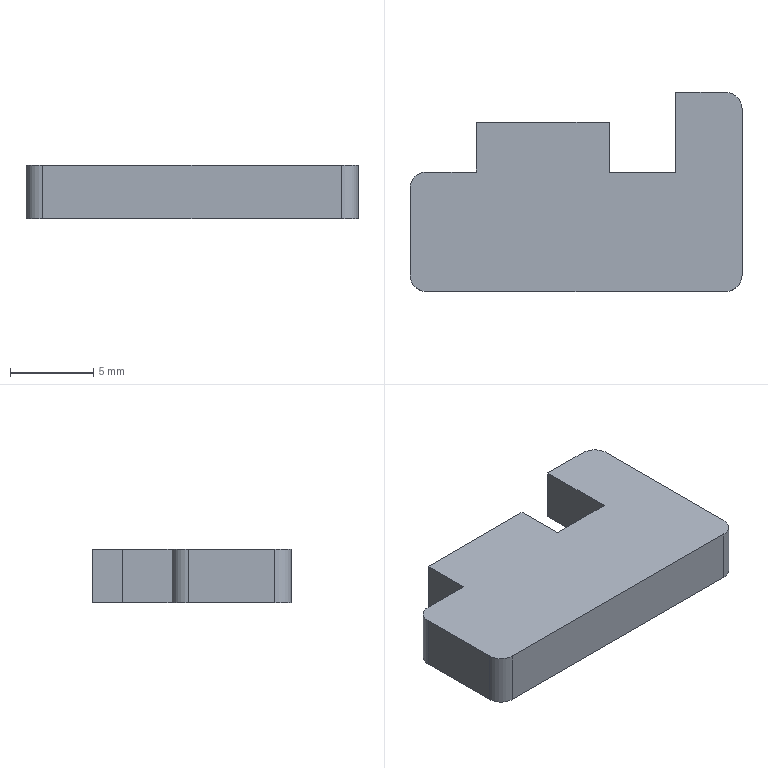Part | SolidWorks | features FlatPattern 1, SMBaseFlange 1, SheetMetal 1 | 1 solid | 16 faces | box 20 x 12 x 3.2 mm | volume 596.293 mm3 | plane 12 | cylinder 4 | commonest cylinder face diameters 2 x4
STEP:
#1=CARTESIAN_POINT('',(7.294,-19.84,0.));
#2=VERTEX_POINT('',#1);
#3=CARTESIAN_POINT('',(4.294,-19.84,0.));
#4=VERTEX_POINT('',#3);
#5=CARTESIAN_POINT('',(7.294,-19.84,0.));
#6=DIRECTION('',(-1.,0.,0.));
#7=VECTOR('',#6,1000.);
#8=LINE('',#5,#7);
#9=EDGE_CURVE('',#2,#4,#8,.T.);
#10=ORIENTED_EDGE('',*,*,#9,.F.);
#11=CARTESIAN_POINT('',(7.294,-19.84,-3.2));
#12=VERTEX_POINT('',#11);
#13=CARTESIAN_POINT('',(7.294,-19.84,-3.2));
#14=DIRECTION('',(0.,0.,1.));
#15=VECTOR('',#14,1000.);
#16=LINE('',#13,#15);
#17=EDGE_CURVE('',#12,#2,#16,.T.);
#18=ORIENTED_EDGE('',*,*,#17,.F.);
#19=CARTESIAN_POINT('',(4.294,-19.84,-3.2));
#20=VERTEX_POINT('',#19);
#21=CARTESIAN_POINT('',(7.294,-19.84,-3.2));
#22=DIRECTION('',(-1.,0.,0.));
#23=VECTOR('',#22,1000.);
#24=LINE('',#21,#23);
#25=EDGE_CURVE('',#12,#20,#24,.T.);
#26=ORIENTED_EDGE('',*,*,#25,.T.);
#27=CARTESIAN_POINT('',(4.294,-19.84,-3.2));
#28=DIRECTION('',(0.,0.,1.));
#29=VECTOR('',#28,1000.);
#30=LINE('',#27,#29);
#31=EDGE_CURVE('',#20,#4,#30,.T.);
#32=ORIENTED_EDGE('',*,*,#31,.T.);
#33=EDGE_LOOP('',(#10,#18,#26,#32));
#34=FACE_OUTER_BOUND('',#33,.T.);
#35=CARTESIAN_POINT('',(7.294,-19.84,-3.2));
#36=DIRECTION('',(0.,1.,0.));
#37=DIRECTION('',(-1.,0.,0.));
#38=AXIS2_PLACEMENT_3D('',#35,#36,#37);
#39=PLANE('',#38);
#40=ADVANCED_FACE('',(#34),#39,.T.);
#41=CARTESIAN_POINT('',(7.294,-16.84,0.));
#42=VERTEX_POINT('',#41);
#43=CARTESIAN_POINT('',(7.294,-19.84,0.));
#44=DIRECTION('',(0.,-1.,0.));
#45=VECTOR('',#44,1000.);
#46=LINE('',#43,#45);
#47=EDGE_CURVE('',#42,#2,#46,.T.);
#48=ORIENTED_EDGE('',*,*,#47,.F.);
#49=CARTESIAN_POINT('',(7.294,-16.84,-3.2));
#50=VERTEX_POINT('',#49);
#51=CARTESIAN_POINT('',(7.294,-16.84,-3.2));
#52=DIRECTION('',(0.,0.,1.));
#53=VECTOR('',#52,1000.);
#54=LINE('',#51,#53);
#55=EDGE_CURVE('',#50,#42,#54,.T.);
#56=ORIENTED_EDGE('',*,*,#55,.F.);
#57=CARTESIAN_POINT('',(7.294,-19.84,-3.2));
#58=DIRECTION('',(0.,-1.,0.));
#59=VECTOR('',#58,1000.);
#60=LINE('',#57,#59);
#61=EDGE_CURVE('',#50,#12,#60,.T.);
#62=ORIENTED_EDGE('',*,*,#61,.T.);
#63=ORIENTED_EDGE('',*,*,#17,.T.);
#64=EDGE_LOOP('',(#48,#56,#62,#63));
#65=FACE_OUTER_BOUND('',#64,.T.);
#66=CARTESIAN_POINT('',(7.294,-19.84,-3.2));
#67=DIRECTION('',(-1.,0.,0.));
#68=DIRECTION('',(0.,-1.,0.));
#69=AXIS2_PLACEMENT_3D('',#66,#67,#68);
#70=PLANE('',#69);
#71=ADVANCED_FACE('',(#65),#70,.T.);
#72=CARTESIAN_POINT('',(15.294,-16.84,0.));
#73=VERTEX_POINT('',#72);
#74=CARTESIAN_POINT('',(7.294,-16.84,0.));
#75=DIRECTION('',(-1.,0.,0.));
#76=VECTOR('',#75,1000.);
#77=LINE('',#74,#76);
#78=EDGE_CURVE('',#73,#42,#77,.T.);
#79=ORIENTED_EDGE('',*,*,#78,.F.);
#80=CARTESIAN_POINT('',(15.294,-16.84,-3.2));
#81=VERTEX_POINT('',#80);
#82=CARTESIAN_POINT('',(15.294,-16.84,-3.2));
#83=DIRECTION('',(0.,0.,1.));
#84=VECTOR('',#83,1000.);
#85=LINE('',#82,#84);
#86=EDGE_CURVE('',#81,#73,#85,.T.);
#87=ORIENTED_EDGE('',*,*,#86,.F.);
#88=CARTESIAN_POINT('',(7.294,-16.84,-3.2));
#89=DIRECTION('',(-1.,0.,0.));
#90=VECTOR('',#89,1000.);
#91=LINE('',#88,#90);
#92=EDGE_CURVE('',#81,#50,#91,.T.);
#93=ORIENTED_EDGE('',*,*,#92,.T.);
#94=ORIENTED_EDGE('',*,*,#55,.T.);
#95=EDGE_LOOP('',(#79,#87,#93,#94));
#96=FACE_OUTER_BOUND('',#95,.T.);
#97=CARTESIAN_POINT('',(7.294,-16.84,-3.2));
#98=DIRECTION('',(0.,1.,0.));
#99=DIRECTION('',(0.,0.,1.));
#100=AXIS2_PLACEMENT_3D('',#97,#98,#99);
#101=PLANE('',#100);
#102=ADVANCED_FACE('',(#96),#101,.T.);
#103=CARTESIAN_POINT('',(15.294,-19.84,0.));
#104=VERTEX_POINT('',#103);
#105=CARTESIAN_POINT('',(15.294,-16.84,0.));
#106=DIRECTION('',(0.,1.,0.));
#107=VECTOR('',#106,1000.);
#108=LINE('',#105,#107);
#109=EDGE_CURVE('',#104,#73,#108,.T.);
#110=ORIENTED_EDGE('',*,*,#109,.F.);
#111=CARTESIAN_POINT('',(15.294,-19.84,-3.2));
#112=VERTEX_POINT('',#111);
#113=CARTESIAN_POINT('',(15.294,-19.84,-3.2));
#114=DIRECTION('',(0.,0.,1.));
#115=VECTOR('',#114,1000.);
#116=LINE('',#113,#115);
#117=EDGE_CURVE('',#112,#104,#116,.T.);
#118=ORIENTED_EDGE('',*,*,#117,.F.);
#119=CARTESIAN_POINT('',(15.294,-16.84,-3.2));
#120=DIRECTION('',(0.,1.,0.));
#121=VECTOR('',#120,1000.);
#122=LINE('',#119,#121);
#123=EDGE_CURVE('',#112,#81,#122,.T.);
#124=ORIENTED_EDGE('',*,*,#123,.T.);
#125=ORIENTED_EDGE('',*,*,#86,.T.);
#126=EDGE_LOOP('',(#110,#118,#124,#125));
#127=FACE_OUTER_BOUND('',#126,.T.);
#128=CARTESIAN_POINT('',(15.294,-16.84,-3.2));
#129=DIRECTION('',(1.,0.,0.));
#130=DIRECTION('',(0.,1.,0.));
#131=AXIS2_PLACEMENT_3D('',#128,#129,#130);
#132=PLANE('',#131);
#133=ADVANCED_FACE('',(#127),#132,.T.);
#134=CARTESIAN_POINT('',(19.294,-19.84,0.));
#135=VERTEX_POINT('',#134);
#136=CARTESIAN_POINT('',(19.294,-19.84,0.));
#137=DIRECTION('',(-1.,0.,0.));
#138=VECTOR('',#137,1000.);
#139=LINE('',#136,#138);
#140=EDGE_CURVE('',#135,#104,#139,.T.);
#141=ORIENTED_EDGE('',*,*,#140,.F.);
#142=CARTESIAN_POINT('',(19.294,-19.84,-3.2));
#143=VERTEX_POINT('',#142);
#144=CARTESIAN_POINT('',(19.294,-19.84,-3.2));
#145=DIRECTION('',(0.,0.,1.));
#146=VECTOR('',#145,1000.);
#147=LINE('',#144,#146);
#148=EDGE_CURVE('',#143,#135,#147,.T.);
#149=ORIENTED_EDGE('',*,*,#148,.F.);
#150=CARTESIAN_POINT('',(19.294,-19.84,-3.2));
#151=DIRECTION('',(-1.,0.,0.));
#152=VECTOR('',#151,1000.);
#153=LINE('',#150,#152);
#154=EDGE_CURVE('',#143,#112,#153,.T.);
#155=ORIENTED_EDGE('',*,*,#154,.T.);
#156=ORIENTED_EDGE('',*,*,#117,.T.);
#157=EDGE_LOOP('',(#141,#149,#155,#156));
#158=FACE_OUTER_BOUND('',#157,.T.);
#159=CARTESIAN_POINT('',(19.294,-19.84,-3.2));
#160=DIRECTION('',(0.,1.,0.));
#161=DIRECTION('',(-1.,0.,0.));
#162=AXIS2_PLACEMENT_3D('',#159,#160,#161);
#163=PLANE('',#162);
#164=ADVANCED_FACE('',(#158),#163,.T.);
#165=CARTESIAN_POINT('',(19.294,-15.04,0.));
#166=VERTEX_POINT('',#165);
#167=CARTESIAN_POINT('',(19.294,-19.84,0.));
#168=DIRECTION('',(0.,-1.,0.));
#169=VECTOR('',#168,1000.);
#170=LINE('',#167,#169);
#171=EDGE_CURVE('',#166,#135,#170,.T.);
#172=ORIENTED_EDGE('',*,*,#171,.F.);
#173=CARTESIAN_POINT('',(19.294,-15.04,-3.2));
#174=VERTEX_POINT('',#173);
#175=CARTESIAN_POINT('',(19.294,-15.04,-3.2));
#176=DIRECTION('',(0.,0.,1.));
#177=VECTOR('',#176,1000.);
#178=LINE('',#175,#177);
#179=EDGE_CURVE('',#174,#166,#178,.T.);
#180=ORIENTED_EDGE('',*,*,#179,.F.);
#181=CARTESIAN_POINT('',(19.294,-19.84,-3.2));
#182=DIRECTION('',(0.,-1.,0.));
#183=VECTOR('',#182,1000.);
#184=LINE('',#181,#183);
#185=EDGE_CURVE('',#174,#143,#184,.T.);
#186=ORIENTED_EDGE('',*,*,#185,.T.);
#187=ORIENTED_EDGE('',*,*,#148,.T.);
#188=EDGE_LOOP('',(#172,#180,#186,#187));
#189=FACE_OUTER_BOUND('',#188,.T.);
#190=CARTESIAN_POINT('',(19.294,-19.84,-3.2));
#191=DIRECTION('',(-1.,0.,0.));
#192=DIRECTION('',(0.,-1.,0.));
#193=AXIS2_PLACEMENT_3D('',#190,#191,#192);
#194=PLANE('',#193);
#195=ADVANCED_FACE('',(#189),#194,.T.);
#196=CARTESIAN_POINT('',(22.294,-15.04,0.));
#197=VERTEX_POINT('',#196);
#198=CARTESIAN_POINT('',(19.294,-15.04,0.));
#199=DIRECTION('',(-1.,0.,0.));
#200=VECTOR('',#199,1000.);
#201=LINE('',#198,#200);
#202=EDGE_CURVE('',#197,#166,#201,.T.);
#203=ORIENTED_EDGE('',*,*,#202,.F.);
#204=CARTESIAN_POINT('',(22.294,-15.04,-3.2));
#205=VERTEX_POINT('',#204);
#206=CARTESIAN_POINT('',(22.294,-15.04,-3.2));
#207=DIRECTION('',(0.,0.,1.));
#208=VECTOR('',#207,1000.);
#209=LINE('',#206,#208);
#210=EDGE_CURVE('',#205,#197,#209,.T.);
#211=ORIENTED_EDGE('',*,*,#210,.F.);
#212=CARTESIAN_POINT('',(19.294,-15.04,-3.2));
#213=DIRECTION('',(-1.,0.,0.));
#214=VECTOR('',#213,1000.);
#215=LINE('',#212,#214);
#216=EDGE_CURVE('',#205,#174,#215,.T.);
#217=ORIENTED_EDGE('',*,*,#216,.T.);
#218=ORIENTED_EDGE('',*,*,#179,.T.);
#219=EDGE_LOOP('',(#203,#211,#217,#218));
#220=FACE_OUTER_BOUND('',#219,.T.);
#221=CARTESIAN_POINT('',(19.294,-15.04,-3.2));
#222=DIRECTION('',(0.,1.,0.));
#223=DIRECTION('',(0.,0.,1.));
#224=AXIS2_PLACEMENT_3D('',#221,#222,#223);
#225=PLANE('',#224);
#226=ADVANCED_FACE('',(#220),#225,.T.);
#227=CARTESIAN_POINT('',(23.294,-16.04,0.));
#228=VERTEX_POINT('',#227);
#229=CARTESIAN_POINT('',(22.294,-16.04,0.));
#230=DIRECTION('',(0.,0.,1.));
#231=DIRECTION('',(-1.,0.,0.));
#232=AXIS2_PLACEMENT_3D('',#229,#230,#231);
#233=CIRCLE('',#232,1.);
#234=EDGE_CURVE('',#228,#197,#233,.T.);
#235=ORIENTED_EDGE('',*,*,#234,.F.);
#236=CARTESIAN_POINT('',(23.294,-16.04,-3.2));
#237=VERTEX_POINT('',#236);
#238=CARTESIAN_POINT('',(23.294,-16.04,-3.2));
#239=DIRECTION('',(0.,0.,1.));
#240=VECTOR('',#239,1000.);
#241=LINE('',#238,#240);
#242=EDGE_CURVE('',#237,#228,#241,.T.);
#243=ORIENTED_EDGE('',*,*,#242,.F.);
#244=CARTESIAN_POINT('',(22.294,-16.04,-3.2));
#245=DIRECTION('',(0.,0.,1.));
#246=DIRECTION('',(-1.,0.,0.));
#247=AXIS2_PLACEMENT_3D('',#244,#245,#246);
#248=CIRCLE('',#247,1.);
#249=EDGE_CURVE('',#237,#205,#248,.T.);
#250=ORIENTED_EDGE('',*,*,#249,.T.);
#251=ORIENTED_EDGE('',*,*,#210,.T.);
#252=EDGE_LOOP('',(#235,#243,#250,#251));
#253=FACE_OUTER_BOUND('',#252,.T.);
#254=CARTESIAN_POINT('',(22.294,-16.04,-3.2));
#255=DIRECTION('',(0.,0.,1.));
#256=DIRECTION('',(1.,0.,0.));
#257=AXIS2_PLACEMENT_3D('',#254,#255,#256);
#258=CYLINDRICAL_SURFACE('',#257,1.);
#259=ADVANCED_FACE('',(#253),#258,.T.);
#260=CARTESIAN_POINT('',(23.294,-26.04,0.));
#261=VERTEX_POINT('',#260);
#262=CARTESIAN_POINT('',(23.294,-16.04,0.));
#263=DIRECTION('',(0.,1.,0.));
#264=VECTOR('',#263,1000.);
#265=LINE('',#262,#264);
#266=EDGE_CURVE('',#261,#228,#265,.T.);
#267=ORIENTED_EDGE('',*,*,#266,.F.);
#268=CARTESIAN_POINT('',(23.294,-26.04,-3.2));
#269=VERTEX_POINT('',#268);
#270=CARTESIAN_POINT('',(23.294,-26.04,-3.2));
#271=DIRECTION('',(0.,0.,1.));
#272=VECTOR('',#271,1000.);
#273=LINE('',#270,#272);
#274=EDGE_CURVE('',#269,#261,#273,.T.);
#275=ORIENTED_EDGE('',*,*,#274,.F.);
#276=CARTESIAN_POINT('',(23.294,-16.04,-3.2));
#277=DIRECTION('',(0.,1.,0.));
#278=VECTOR('',#277,1000.);
#279=LINE('',#276,#278);
#280=EDGE_CURVE('',#269,#237,#279,.T.);
#281=ORIENTED_EDGE('',*,*,#280,.T.);
#282=ORIENTED_EDGE('',*,*,#242,.T.);
#283=EDGE_LOOP('',(#267,#275,#281,#282));
#284=FACE_OUTER_BOUND('',#283,.T.);
#285=CARTESIAN_POINT('',(23.294,-16.04,-3.2));
#286=DIRECTION('',(1.,0.,0.));
#287=DIRECTION('',(0.,0.,-1.));
#288=AXIS2_PLACEMENT_3D('',#285,#286,#287);
#289=PLANE('',#288);
#290=ADVANCED_FACE('',(#284),#289,.T.);
#291=CARTESIAN_POINT('',(22.294,-27.04,0.));
#292=VERTEX_POINT('',#291);
#293=CARTESIAN_POINT('',(22.294,-26.04,0.));
#294=DIRECTION('',(0.,0.,1.));
#295=DIRECTION('',(-1.,0.,0.));
#296=AXIS2_PLACEMENT_3D('',#293,#294,#295);
#297=CIRCLE('',#296,1.);
#298=EDGE_CURVE('',#292,#261,#297,.T.);
#299=ORIENTED_EDGE('',*,*,#298,.F.);
#300=CARTESIAN_POINT('',(22.294,-27.04,-3.2));
#301=VERTEX_POINT('',#300);
#302=CARTESIAN_POINT('',(22.294,-27.04,-3.2));
#303=DIRECTION('',(0.,0.,1.));
#304=VECTOR('',#303,1000.);
#305=LINE('',#302,#304);
#306=EDGE_CURVE('',#301,#292,#305,.T.);
#307=ORIENTED_EDGE('',*,*,#306,.F.);
#308=CARTESIAN_POINT('',(22.294,-26.04,-3.2));
#309=DIRECTION('',(0.,0.,1.));
#310=DIRECTION('',(-1.,0.,0.));
#311=AXIS2_PLACEMENT_3D('',#308,#309,#310);
#312=CIRCLE('',#311,1.);
#313=EDGE_CURVE('',#301,#269,#312,.T.);
#314=ORIENTED_EDGE('',*,*,#313,.T.);
#315=ORIENTED_EDGE('',*,*,#274,.T.);
#316=EDGE_LOOP('',(#299,#307,#314,#315));
#317=FACE_OUTER_BOUND('',#316,.T.);
#318=CARTESIAN_POINT('',(22.294,-26.04,-3.2));
#319=DIRECTION('',(0.,0.,1.));
#320=DIRECTION('',(1.,0.,0.));
#321=AXIS2_PLACEMENT_3D('',#318,#319,#320);
#322=CYLINDRICAL_SURFACE('',#321,1.);
#323=ADVANCED_FACE('',(#317),#322,.T.);
#324=CARTESIAN_POINT('',(4.294,-27.04,0.));
#325=VERTEX_POINT('',#324);
#326=CARTESIAN_POINT('',(22.294,-27.04,0.));
#327=DIRECTION('',(1.,0.,0.));
#328=VECTOR('',#327,1000.);
#329=LINE('',#326,#328);
#330=EDGE_CURVE('',#325,#292,#329,.T.);
#331=ORIENTED_EDGE('',*,*,#330,.F.);
#332=CARTESIAN_POINT('',(4.294,-27.04,-3.2));
#333=VERTEX_POINT('',#332);
#334=CARTESIAN_POINT('',(4.294,-27.04,-3.2));
#335=DIRECTION('',(0.,0.,1.));
#336=VECTOR('',#335,1000.);
#337=LINE('',#334,#336);
#338=EDGE_CURVE('',#333,#325,#337,.T.);
#339=ORIENTED_EDGE('',*,*,#338,.F.);
#340=CARTESIAN_POINT('',(22.294,-27.04,-3.2));
#341=DIRECTION('',(1.,0.,0.));
#342=VECTOR('',#341,1000.);
#343=LINE('',#340,#342);
#344=EDGE_CURVE('',#333,#301,#343,.T.);
#345=ORIENTED_EDGE('',*,*,#344,.T.);
#346=ORIENTED_EDGE('',*,*,#306,.T.);
#347=EDGE_LOOP('',(#331,#339,#345,#346));
#348=FACE_OUTER_BOUND('',#347,.T.);
#349=CARTESIAN_POINT('',(22.294,-27.04,-3.2));
#350=DIRECTION('',(0.,-1.,0.));
#351=DIRECTION('',(0.,0.,-1.));
#352=AXIS2_PLACEMENT_3D('',#349,#350,#351);
#353=PLANE('',#352);
#354=ADVANCED_FACE('',(#348),#353,.T.);
#355=CARTESIAN_POINT('',(3.294,-26.04,0.));
#356=VERTEX_POINT('',#355);
#357=CARTESIAN_POINT('',(4.294,-26.04,0.));
#358=DIRECTION('',(0.,0.,1.));
#359=DIRECTION('',(-1.,0.,0.));
#360=AXIS2_PLACEMENT_3D('',#357,#358,#359);
#361=CIRCLE('',#360,1.);
#362=EDGE_CURVE('',#356,#325,#361,.T.);
#363=ORIENTED_EDGE('',*,*,#362,.F.);
#364=CARTESIAN_POINT('',(3.294,-26.04,-3.2));
#365=VERTEX_POINT('',#364);
#366=CARTESIAN_POINT('',(3.294,-26.04,-3.2));
#367=DIRECTION('',(0.,0.,1.));
#368=VECTOR('',#367,1000.);
#369=LINE('',#366,#368);
#370=EDGE_CURVE('',#365,#356,#369,.T.);
#371=ORIENTED_EDGE('',*,*,#370,.F.);
#372=CARTESIAN_POINT('',(4.294,-26.04,-3.2));
#373=DIRECTION('',(0.,0.,1.));
#374=DIRECTION('',(-1.,0.,0.));
#375=AXIS2_PLACEMENT_3D('',#372,#373,#374);
#376=CIRCLE('',#375,1.);
#377=EDGE_CURVE('',#365,#333,#376,.T.);
#378=ORIENTED_EDGE('',*,*,#377,.T.);
#379=ORIENTED_EDGE('',*,*,#338,.T.);
#380=EDGE_LOOP('',(#363,#371,#378,#379));
#381=FACE_OUTER_BOUND('',#380,.T.);
#382=CARTESIAN_POINT('',(4.294,-26.04,-3.2));
#383=DIRECTION('',(0.,0.,1.));
#384=DIRECTION('',(1.,0.,0.));
#385=AXIS2_PLACEMENT_3D('',#382,#383,#384);
#386=CYLINDRICAL_SURFACE('',#385,1.);
#387=ADVANCED_FACE('',(#381),#386,.T.);
#388=CARTESIAN_POINT('',(3.294,-20.84,0.));
#389=VERTEX_POINT('',#388);
#390=CARTESIAN_POINT('',(3.294,-26.04,0.));
#391=DIRECTION('',(0.,-1.,0.));
#392=VECTOR('',#391,1000.);
#393=LINE('',#390,#392);
#394=EDGE_CURVE('',#389,#356,#393,.T.);
#395=ORIENTED_EDGE('',*,*,#394,.F.);
#396=CARTESIAN_POINT('',(3.294,-20.84,-3.2));
#397=VERTEX_POINT('',#396);
#398=CARTESIAN_POINT('',(3.294,-20.84,-3.2));
#399=DIRECTION('',(0.,0.,1.));
#400=VECTOR('',#399,1000.);
#401=LINE('',#398,#400);
#402=EDGE_CURVE('',#397,#389,#401,.T.);
#403=ORIENTED_EDGE('',*,*,#402,.F.);
#404=CARTESIAN_POINT('',(3.294,-26.04,-3.2));
#405=DIRECTION('',(0.,-1.,0.));
#406=VECTOR('',#405,1000.);
#407=LINE('',#404,#406);
#408=EDGE_CURVE('',#397,#365,#407,.T.);
#409=ORIENTED_EDGE('',*,*,#408,.T.);
#410=ORIENTED_EDGE('',*,*,#370,.T.);
#411=EDGE_LOOP('',(#395,#403,#409,#410));
#412=FACE_OUTER_BOUND('',#411,.T.);
#413=CARTESIAN_POINT('',(3.294,-26.04,-3.2));
#414=DIRECTION('',(-1.,0.,0.));
#415=DIRECTION('',(0.,-1.,0.));
#416=AXIS2_PLACEMENT_3D('',#413,#414,#415);
#417=PLANE('',#416);
#418=ADVANCED_FACE('',(#412),#417,.T.);
#419=CARTESIAN_POINT('',(4.294,-20.84,0.));
#420=DIRECTION('',(0.,0.,1.));
#421=DIRECTION('',(1.,0.,0.));
#422=AXIS2_PLACEMENT_3D('',#419,#420,#421);
#423=CIRCLE('',#422,1.);
#424=EDGE_CURVE('',#4,#389,#423,.T.);
#425=ORIENTED_EDGE('',*,*,#424,.F.);
#426=ORIENTED_EDGE('',*,*,#31,.F.);
#427=CARTESIAN_POINT('',(4.294,-20.84,-3.2));
#428=DIRECTION('',(0.,0.,1.));
#429=DIRECTION('',(1.,0.,0.));
#430=AXIS2_PLACEMENT_3D('',#427,#428,#429);
#431=CIRCLE('',#430,1.);
#432=EDGE_CURVE('',#20,#397,#431,.T.);
#433=ORIENTED_EDGE('',*,*,#432,.T.);
#434=ORIENTED_EDGE('',*,*,#402,.T.);
#435=EDGE_LOOP('',(#425,#426,#433,#434));
#436=FACE_OUTER_BOUND('',#435,.T.);
#437=CARTESIAN_POINT('',(4.294,-20.84,-3.2));
#438=DIRECTION('',(0.,0.,1.));
#439=DIRECTION('',(1.,0.,0.));
#440=AXIS2_PLACEMENT_3D('',#437,#438,#439);
#441=CYLINDRICAL_SURFACE('',#440,1.);
#442=ADVANCED_FACE('',(#436),#441,.T.);
#443=ORIENTED_EDGE('',*,*,#25,.F.);
#444=ORIENTED_EDGE('',*,*,#61,.F.);
#445=ORIENTED_EDGE('',*,*,#92,.F.);
#446=ORIENTED_EDGE('',*,*,#123,.F.);
#447=ORIENTED_EDGE('',*,*,#154,.F.);
#448=ORIENTED_EDGE('',*,*,#185,.F.);
#449=ORIENTED_EDGE('',*,*,#216,.F.);
#450=ORIENTED_EDGE('',*,*,#249,.F.);
#451=ORIENTED_EDGE('',*,*,#280,.F.);
#452=ORIENTED_EDGE('',*,*,#313,.F.);
#453=ORIENTED_EDGE('',*,*,#344,.F.);
#454=ORIENTED_EDGE('',*,*,#377,.F.);
#455=ORIENTED_EDGE('',*,*,#408,.F.);
#456=ORIENTED_EDGE('',*,*,#432,.F.);
#457=EDGE_LOOP('',(#443,#444,#445,#446,#447,#448,#449,#450,#451,#452,#453,#454,#455,#456));
#458=FACE_OUTER_BOUND('',#457,.T.);
#459=CARTESIAN_POINT('',(4.294,-20.84,-3.2));
#460=DIRECTION('',(0.,0.,1.));
#461=DIRECTION('',(1.,0.,0.));
#462=AXIS2_PLACEMENT_3D('',#459,#460,#461);
#463=PLANE('',#462);
#464=ADVANCED_FACE('',(#458),#463,.F.);
#465=ORIENTED_EDGE('',*,*,#9,.T.);
#466=ORIENTED_EDGE('',*,*,#424,.T.);
#467=ORIENTED_EDGE('',*,*,#394,.T.);
#468=ORIENTED_EDGE('',*,*,#362,.T.);
#469=ORIENTED_EDGE('',*,*,#330,.T.);
#470=ORIENTED_EDGE('',*,*,#298,.T.);
#471=ORIENTED_EDGE('',*,*,#266,.T.);
#472=ORIENTED_EDGE('',*,*,#234,.T.);
#473=ORIENTED_EDGE('',*,*,#202,.T.);
#474=ORIENTED_EDGE('',*,*,#171,.T.);
#475=ORIENTED_EDGE('',*,*,#140,.T.);
#476=ORIENTED_EDGE('',*,*,#109,.T.);
#477=ORIENTED_EDGE('',*,*,#78,.T.);
#478=ORIENTED_EDGE('',*,*,#47,.T.);
#479=EDGE_LOOP('',(#465,#466,#467,#468,#469,#470,#471,#472,#473,#474,#475,#476,#477,#478));
#480=FACE_OUTER_BOUND('',#479,.T.);
#481=CARTESIAN_POINT('',(4.294,-20.84,0.));
#482=DIRECTION('',(0.,0.,1.));
#483=DIRECTION('',(1.,0.,0.));
#484=AXIS2_PLACEMENT_3D('',#481,#482,#483);
#485=PLANE('',#484);
#486=ADVANCED_FACE('',(#480),#485,.T.);
#487=CLOSED_SHELL('',(#40,#71,#102,#133,#164,#195,#226,#259,#290,#323,#354,#387,#418,#442,#464,#486));
#488=MANIFOLD_SOLID_BREP('',#487);
#489=CARTESIAN_POINT('',(0.,0.,0.));
#490=DIRECTION('',(0.,0.,1.));
#491=DIRECTION('',(1.,0.,0.));
#492=AXIS2_PLACEMENT_3D('',#489,#490,#491);
#493=(LENGTH_UNIT()NAMED_UNIT(*)SI_UNIT(.MILLI.,.METRE.));
#494=UNCERTAINTY_MEASURE_WITH_UNIT(LENGTH_MEASURE(0.00001),#493,'','');
#495=(NAMED_UNIT(*)PLANE_ANGLE_UNIT()SI_UNIT($,.RADIAN.));
#496=(NAMED_UNIT(*)SI_UNIT($,.STERADIAN.)SOLID_ANGLE_UNIT());
#497=(GEOMETRIC_REPRESENTATION_CONTEXT(3)GLOBAL_UNCERTAINTY_ASSIGNED_CONTEXT((#494))GLOBAL_UNIT_ASSIGNED_CONTEXT((#493,#495,#496))REPRESENTATION_CONTEXT('',''));
#498=ADVANCED_BREP_SHAPE_REPRESENTATION('',(#488,#492),#497);